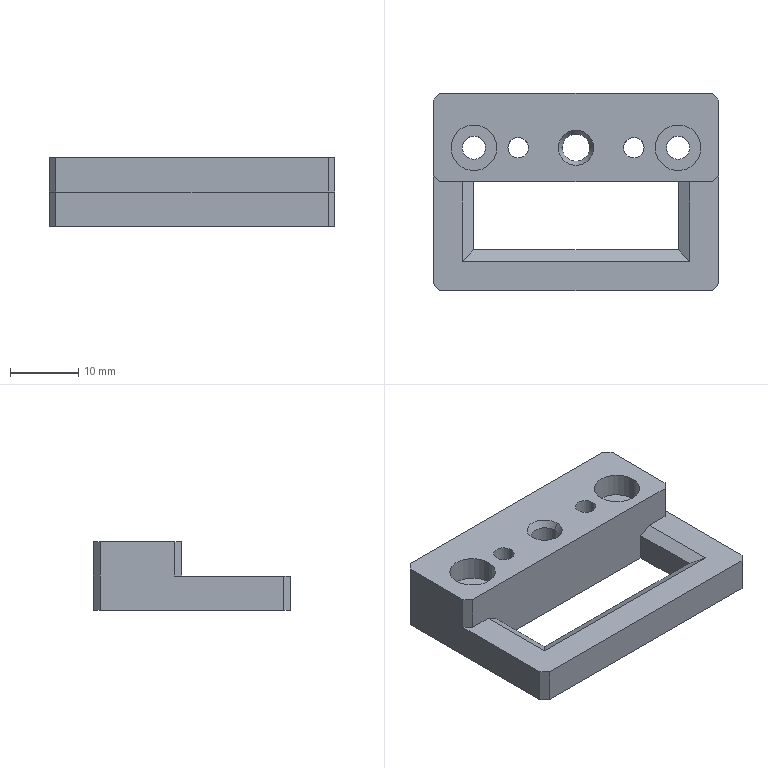Part | NX | features BREP 1 | 1 solid | 38 faces | box 42 x 29 x 10 mm | volume 6619 mm3 | plane 22 | cylinder 14 | cone 2 | commonest cylinder face diameters 3 x4 3.4 x4 6.7 x4 4 x2
STEP:
#1=CARTESIAN_POINT('',(-2.,0.,-1.));
#2=VERTEX_POINT('',#1);
#3=CARTESIAN_POINT('',(2.,0.,-1.));
#4=VERTEX_POINT('',#3);
#5=CARTESIAN_POINT('',(0.,0.,-1.));
#6=DIRECTION('',(0.,0.,1.));
#7=DIRECTION('',(1.,0.,0.));
#8=AXIS2_PLACEMENT_3D('',#5,#6,#7);
#9=CIRCLE('',#8,2.);
#10=EDGE_CURVE('',#2,#4,#9,.T.);
#11=ORIENTED_EDGE('',*,*,#10,.F.);
#12=CARTESIAN_POINT('',(-2.577,0.,0.));
#13=VERTEX_POINT('',#12);
#14=CARTESIAN_POINT('',(-2.,0.,-1.));
#15=DIRECTION('',(-0.5,0.,0.866));
#16=VECTOR('',#15,1000.);
#17=LINE('',#14,#16);
#18=EDGE_CURVE('',#13,#2,#17,.F.);
#19=ORIENTED_EDGE('',*,*,#18,.F.);
#20=CARTESIAN_POINT('',(2.577,0.,0.));
#21=VERTEX_POINT('',#20);
#22=CARTESIAN_POINT('',(0.,0.,0.));
#23=DIRECTION('',(0.,0.,-1.));
#24=DIRECTION('',(1.,0.,0.));
#25=AXIS2_PLACEMENT_3D('',#22,#23,#24);
#26=CIRCLE('',#25,2.577);
#27=EDGE_CURVE('',#21,#13,#26,.T.);
#28=ORIENTED_EDGE('',*,*,#27,.F.);
#29=CARTESIAN_POINT('',(2.,0.,-1.));
#30=DIRECTION('',(0.5,0.,0.866));
#31=VECTOR('',#30,1000.);
#32=LINE('',#29,#31);
#33=EDGE_CURVE('',#21,#4,#32,.F.);
#34=ORIENTED_EDGE('',*,*,#33,.T.);
#35=EDGE_LOOP('',(#11,#19,#28,#34));
#36=FACE_BOUND('',#35,.T.);
#37=CARTESIAN_POINT('',(0.,0.,-1.));
#38=DIRECTION('',(0.,0.,1.));
#39=DIRECTION('',(1.,0.,0.));
#40=AXIS2_PLACEMENT_3D('',#37,#38,#39);
#41=CONICAL_SURFACE('',#40,2.,0.5236);
#42=ADVANCED_FACE('',(#36),#41,.F.);
#43=CARTESIAN_POINT('',(-2.,0.,-10.));
#44=VERTEX_POINT('',#43);
#45=CARTESIAN_POINT('',(2.,0.,-10.));
#46=VERTEX_POINT('',#45);
#47=CARTESIAN_POINT('',(0.,0.,-10.));
#48=DIRECTION('',(0.,0.,1.));
#49=DIRECTION('',(1.,0.,0.));
#50=AXIS2_PLACEMENT_3D('',#47,#48,#49);
#51=CIRCLE('',#50,2.);
#52=EDGE_CURVE('',#44,#46,#51,.T.);
#53=ORIENTED_EDGE('',*,*,#52,.F.);
#54=CARTESIAN_POINT('',(-2.,0.,-29.));
#55=DIRECTION('',(0.,0.,1.));
#56=VECTOR('',#55,1000.);
#57=LINE('',#54,#56);
#58=EDGE_CURVE('',#2,#44,#57,.F.);
#59=ORIENTED_EDGE('',*,*,#58,.F.);
#60=ORIENTED_EDGE('',*,*,#10,.T.);
#61=CARTESIAN_POINT('',(2.,0.,-29.));
#62=DIRECTION('',(0.,0.,1.));
#63=VECTOR('',#62,1000.);
#64=LINE('',#61,#63);
#65=EDGE_CURVE('',#4,#46,#64,.F.);
#66=ORIENTED_EDGE('',*,*,#65,.T.);
#67=EDGE_LOOP('',(#53,#59,#60,#66));
#68=FACE_BOUND('',#67,.T.);
#69=CARTESIAN_POINT('',(0.,0.,-29.));
#70=DIRECTION('',(0.,0.,1.));
#71=DIRECTION('',(1.,0.,0.));
#72=AXIS2_PLACEMENT_3D('',#69,#70,#71);
#73=CYLINDRICAL_SURFACE('',#72,2.);
#74=ADVANCED_FACE('',(#68),#73,.F.);
#75=CARTESIAN_POINT('',(7.,0.,-10.));
#76=VERTEX_POINT('',#75);
#77=CARTESIAN_POINT('',(10.,0.,-10.));
#78=VERTEX_POINT('',#77);
#79=CARTESIAN_POINT('',(8.5,0.,-10.));
#80=DIRECTION('',(0.,0.,1.));
#81=DIRECTION('',(1.,0.,0.));
#82=AXIS2_PLACEMENT_3D('',#79,#80,#81);
#83=CIRCLE('',#82,1.5);
#84=EDGE_CURVE('',#76,#78,#83,.T.);
#85=ORIENTED_EDGE('',*,*,#84,.F.);
#86=CARTESIAN_POINT('',(7.,0.,0.));
#87=VERTEX_POINT('',#86);
#88=CARTESIAN_POINT('',(7.,0.,-19.));
#89=DIRECTION('',(0.,0.,1.));
#90=VECTOR('',#89,1000.);
#91=LINE('',#88,#90);
#92=EDGE_CURVE('',#87,#76,#91,.F.);
#93=ORIENTED_EDGE('',*,*,#92,.F.);
#94=CARTESIAN_POINT('',(10.,0.,0.));
#95=VERTEX_POINT('',#94);
#96=CARTESIAN_POINT('',(8.5,0.,0.));
#97=DIRECTION('',(0.,0.,1.));
#98=DIRECTION('',(1.,0.,0.));
#99=AXIS2_PLACEMENT_3D('',#96,#97,#98);
#100=CIRCLE('',#99,1.5);
#101=EDGE_CURVE('',#87,#95,#100,.T.);
#102=ORIENTED_EDGE('',*,*,#101,.T.);
#103=CARTESIAN_POINT('',(10.,0.,-19.));
#104=DIRECTION('',(0.,0.,1.));
#105=VECTOR('',#104,1000.);
#106=LINE('',#103,#105);
#107=EDGE_CURVE('',#95,#78,#106,.F.);
#108=ORIENTED_EDGE('',*,*,#107,.T.);
#109=EDGE_LOOP('',(#85,#93,#102,#108));
#110=FACE_BOUND('',#109,.T.);
#111=CARTESIAN_POINT('',(8.5,0.,-19.));
#112=DIRECTION('',(0.,0.,1.));
#113=DIRECTION('',(1.,0.,0.));
#114=AXIS2_PLACEMENT_3D('',#111,#112,#113);
#115=CYLINDRICAL_SURFACE('',#114,1.5);
#116=ADVANCED_FACE('',(#110),#115,.F.);
#117=CARTESIAN_POINT('',(-10.,0.,-10.));
#118=VERTEX_POINT('',#117);
#119=CARTESIAN_POINT('',(-7.,0.,-10.));
#120=VERTEX_POINT('',#119);
#121=CARTESIAN_POINT('',(-8.5,0.,-10.));
#122=DIRECTION('',(0.,0.,1.));
#123=DIRECTION('',(1.,0.,0.));
#124=AXIS2_PLACEMENT_3D('',#121,#122,#123);
#125=CIRCLE('',#124,1.5);
#126=EDGE_CURVE('',#118,#120,#125,.T.);
#127=ORIENTED_EDGE('',*,*,#126,.F.);
#128=CARTESIAN_POINT('',(-10.,0.,0.));
#129=VERTEX_POINT('',#128);
#130=CARTESIAN_POINT('',(-10.,0.,-19.));
#131=DIRECTION('',(0.,0.,1.));
#132=VECTOR('',#131,1000.);
#133=LINE('',#130,#132);
#134=EDGE_CURVE('',#129,#118,#133,.F.);
#135=ORIENTED_EDGE('',*,*,#134,.F.);
#136=CARTESIAN_POINT('',(-7.,0.,0.));
#137=VERTEX_POINT('',#136);
#138=CARTESIAN_POINT('',(-8.5,0.,0.));
#139=DIRECTION('',(0.,0.,1.));
#140=DIRECTION('',(1.,0.,0.));
#141=AXIS2_PLACEMENT_3D('',#138,#139,#140);
#142=CIRCLE('',#141,1.5);
#143=EDGE_CURVE('',#129,#137,#142,.T.);
#144=ORIENTED_EDGE('',*,*,#143,.T.);
#145=CARTESIAN_POINT('',(-7.,0.,-19.));
#146=DIRECTION('',(0.,0.,1.));
#147=VECTOR('',#146,1000.);
#148=LINE('',#145,#147);
#149=EDGE_CURVE('',#137,#120,#148,.F.);
#150=ORIENTED_EDGE('',*,*,#149,.T.);
#151=EDGE_LOOP('',(#127,#135,#144,#150));
#152=FACE_BOUND('',#151,.T.);
#153=CARTESIAN_POINT('',(-8.5,0.,-19.));
#154=DIRECTION('',(0.,0.,1.));
#155=DIRECTION('',(1.,0.,0.));
#156=AXIS2_PLACEMENT_3D('',#153,#154,#155);
#157=CYLINDRICAL_SURFACE('',#156,1.5);
#158=ADVANCED_FACE('',(#152),#157,.F.);
#159=CARTESIAN_POINT('',(-18.35,0.,-3.5));
#160=VERTEX_POINT('',#159);
#161=CARTESIAN_POINT('',(-11.65,0.,-3.5));
#162=VERTEX_POINT('',#161);
#163=CARTESIAN_POINT('',(-15.,0.,-3.5));
#164=DIRECTION('',(0.,0.,1.));
#165=DIRECTION('',(1.,0.,0.));
#166=AXIS2_PLACEMENT_3D('',#163,#164,#165);
#167=CIRCLE('',#166,3.35);
#168=EDGE_CURVE('',#160,#162,#167,.T.);
#169=ORIENTED_EDGE('',*,*,#168,.F.);
#170=CARTESIAN_POINT('',(-18.35,0.,0.));
#171=VERTEX_POINT('',#170);
#172=CARTESIAN_POINT('',(-18.35,0.,0.));
#173=DIRECTION('',(0.,0.,1.));
#174=VECTOR('',#173,1000.);
#175=LINE('',#172,#174);
#176=EDGE_CURVE('',#171,#160,#175,.F.);
#177=ORIENTED_EDGE('',*,*,#176,.F.);
#178=CARTESIAN_POINT('',(-11.65,0.,0.));
#179=VERTEX_POINT('',#178);
#180=CARTESIAN_POINT('',(-15.,0.,0.));
#181=DIRECTION('',(0.,0.,1.));
#182=DIRECTION('',(1.,0.,0.));
#183=AXIS2_PLACEMENT_3D('',#180,#181,#182);
#184=CIRCLE('',#183,3.35);
#185=EDGE_CURVE('',#171,#179,#184,.T.);
#186=ORIENTED_EDGE('',*,*,#185,.T.);
#187=CARTESIAN_POINT('',(-11.65,0.,0.));
#188=DIRECTION('',(0.,0.,1.));
#189=VECTOR('',#188,1000.);
#190=LINE('',#187,#189);
#191=EDGE_CURVE('',#179,#162,#190,.F.);
#192=ORIENTED_EDGE('',*,*,#191,.T.);
#193=EDGE_LOOP('',(#169,#177,#186,#192));
#194=FACE_BOUND('',#193,.T.);
#195=CARTESIAN_POINT('',(-15.,0.,0.));
#196=DIRECTION('',(0.,0.,1.));
#197=DIRECTION('',(1.,0.,0.));
#198=AXIS2_PLACEMENT_3D('',#195,#196,#197);
#199=CYLINDRICAL_SURFACE('',#198,3.35);
#200=ADVANCED_FACE('',(#194),#199,.F.);
#201=CARTESIAN_POINT('',(-16.7,0.,-10.));
#202=VERTEX_POINT('',#201);
#203=CARTESIAN_POINT('',(-13.3,0.,-10.));
#204=VERTEX_POINT('',#203);
#205=CARTESIAN_POINT('',(-15.,0.,-10.));
#206=DIRECTION('',(0.,0.,1.));
#207=DIRECTION('',(1.,0.,0.));
#208=AXIS2_PLACEMENT_3D('',#205,#206,#207);
#209=CIRCLE('',#208,1.7);
#210=EDGE_CURVE('',#202,#204,#209,.T.);
#211=ORIENTED_EDGE('',*,*,#210,.F.);
#212=CARTESIAN_POINT('',(-16.7,0.,-3.5));
#213=VERTEX_POINT('',#212);
#214=CARTESIAN_POINT('',(-16.7,0.,0.));
#215=DIRECTION('',(0.,0.,1.));
#216=VECTOR('',#215,1000.);
#217=LINE('',#214,#216);
#218=EDGE_CURVE('',#213,#202,#217,.F.);
#219=ORIENTED_EDGE('',*,*,#218,.F.);
#220=CARTESIAN_POINT('',(-13.3,0.,-3.5));
#221=VERTEX_POINT('',#220);
#222=CARTESIAN_POINT('',(-15.,0.,-3.5));
#223=DIRECTION('',(0.,0.,1.));
#224=DIRECTION('',(1.,0.,0.));
#225=AXIS2_PLACEMENT_3D('',#222,#223,#224);
#226=CIRCLE('',#225,1.7);
#227=EDGE_CURVE('',#213,#221,#226,.T.);
#228=ORIENTED_EDGE('',*,*,#227,.T.);
#229=CARTESIAN_POINT('',(-13.3,0.,0.));
#230=DIRECTION('',(0.,0.,1.));
#231=VECTOR('',#230,1000.);
#232=LINE('',#229,#231);
#233=EDGE_CURVE('',#221,#204,#232,.F.);
#234=ORIENTED_EDGE('',*,*,#233,.T.);
#235=EDGE_LOOP('',(#211,#219,#228,#234));
#236=FACE_BOUND('',#235,.T.);
#237=CARTESIAN_POINT('',(-15.,0.,0.));
#238=DIRECTION('',(0.,0.,1.));
#239=DIRECTION('',(1.,0.,0.));
#240=AXIS2_PLACEMENT_3D('',#237,#238,#239);
#241=CYLINDRICAL_SURFACE('',#240,1.7);
#242=ADVANCED_FACE('',(#236),#241,.F.);
#243=CARTESIAN_POINT('',(11.65,0.,-3.5));
#244=VERTEX_POINT('',#243);
#245=CARTESIAN_POINT('',(18.35,0.,-3.5));
#246=VERTEX_POINT('',#245);
#247=CARTESIAN_POINT('',(15.,0.,-3.5));
#248=DIRECTION('',(0.,0.,1.));
#249=DIRECTION('',(1.,0.,0.));
#250=AXIS2_PLACEMENT_3D('',#247,#248,#249);
#251=CIRCLE('',#250,3.35);
#252=EDGE_CURVE('',#244,#246,#251,.T.);
#253=ORIENTED_EDGE('',*,*,#252,.F.);
#254=CARTESIAN_POINT('',(11.65,0.,0.));
#255=VERTEX_POINT('',#254);
#256=CARTESIAN_POINT('',(11.65,0.,0.));
#257=DIRECTION('',(0.,0.,1.));
#258=VECTOR('',#257,1000.);
#259=LINE('',#256,#258);
#260=EDGE_CURVE('',#255,#244,#259,.F.);
#261=ORIENTED_EDGE('',*,*,#260,.F.);
#262=CARTESIAN_POINT('',(18.35,0.,0.));
#263=VERTEX_POINT('',#262);
#264=CARTESIAN_POINT('',(15.,0.,0.));
#265=DIRECTION('',(0.,0.,1.));
#266=DIRECTION('',(1.,0.,0.));
#267=AXIS2_PLACEMENT_3D('',#264,#265,#266);
#268=CIRCLE('',#267,3.35);
#269=EDGE_CURVE('',#255,#263,#268,.T.);
#270=ORIENTED_EDGE('',*,*,#269,.T.);
#271=CARTESIAN_POINT('',(18.35,0.,0.));
#272=DIRECTION('',(0.,0.,1.));
#273=VECTOR('',#272,1000.);
#274=LINE('',#271,#273);
#275=EDGE_CURVE('',#263,#246,#274,.F.);
#276=ORIENTED_EDGE('',*,*,#275,.T.);
#277=EDGE_LOOP('',(#253,#261,#270,#276));
#278=FACE_BOUND('',#277,.T.);
#279=CARTESIAN_POINT('',(15.,0.,0.));
#280=DIRECTION('',(0.,0.,1.));
#281=DIRECTION('',(1.,0.,0.));
#282=AXIS2_PLACEMENT_3D('',#279,#280,#281);
#283=CYLINDRICAL_SURFACE('',#282,3.35);
#284=ADVANCED_FACE('',(#278),#283,.F.);
#285=CARTESIAN_POINT('',(13.3,0.,-10.));
#286=VERTEX_POINT('',#285);
#287=CARTESIAN_POINT('',(16.7,0.,-10.));
#288=VERTEX_POINT('',#287);
#289=CARTESIAN_POINT('',(15.,0.,-10.));
#290=DIRECTION('',(0.,0.,1.));
#291=DIRECTION('',(1.,0.,0.));
#292=AXIS2_PLACEMENT_3D('',#289,#290,#291);
#293=CIRCLE('',#292,1.7);
#294=EDGE_CURVE('',#286,#288,#293,.T.);
#295=ORIENTED_EDGE('',*,*,#294,.F.);
#296=CARTESIAN_POINT('',(13.3,0.,-3.5));
#297=VERTEX_POINT('',#296);
#298=CARTESIAN_POINT('',(13.3,0.,0.));
#299=DIRECTION('',(0.,0.,1.));
#300=VECTOR('',#299,1000.);
#301=LINE('',#298,#300);
#302=EDGE_CURVE('',#297,#286,#301,.F.);
#303=ORIENTED_EDGE('',*,*,#302,.F.);
#304=CARTESIAN_POINT('',(16.7,0.,-3.5));
#305=VERTEX_POINT('',#304);
#306=CARTESIAN_POINT('',(15.,0.,-3.5));
#307=DIRECTION('',(0.,0.,1.));
#308=DIRECTION('',(1.,0.,0.));
#309=AXIS2_PLACEMENT_3D('',#306,#307,#308);
#310=CIRCLE('',#309,1.7);
#311=EDGE_CURVE('',#297,#305,#310,.T.);
#312=ORIENTED_EDGE('',*,*,#311,.T.);
#313=CARTESIAN_POINT('',(16.7,0.,0.));
#314=DIRECTION('',(0.,0.,1.));
#315=VECTOR('',#314,1000.);
#316=LINE('',#313,#315);
#317=EDGE_CURVE('',#305,#288,#316,.F.);
#318=ORIENTED_EDGE('',*,*,#317,.T.);
#319=EDGE_LOOP('',(#295,#303,#312,#318));
#320=FACE_BOUND('',#319,.T.);
#321=CARTESIAN_POINT('',(15.,0.,0.));
#322=DIRECTION('',(0.,0.,1.));
#323=DIRECTION('',(1.,0.,0.));
#324=AXIS2_PLACEMENT_3D('',#321,#322,#323);
#325=CYLINDRICAL_SURFACE('',#324,1.7);
#326=ADVANCED_FACE('',(#320),#325,.F.);
#327=CARTESIAN_POINT('',(20.,-21.,-10.));
#328=VERTEX_POINT('',#327);
#329=CARTESIAN_POINT('',(20.,-21.,-5.));
#330=VERTEX_POINT('',#329);
#331=CARTESIAN_POINT('',(20.,-21.,0.));
#332=DIRECTION('',(0.,0.,1.));
#333=VECTOR('',#332,1000.);
#334=LINE('',#331,#333);
#335=EDGE_CURVE('',#328,#330,#334,.T.);
#336=ORIENTED_EDGE('',*,*,#335,.T.);
#337=CARTESIAN_POINT('',(-20.,-21.,-5.));
#338=VERTEX_POINT('',#337);
#339=CARTESIAN_POINT('',(0.,-21.,-5.));
#340=DIRECTION('',(-1.,0.,0.));
#341=VECTOR('',#340,1000.);
#342=LINE('',#339,#341);
#343=EDGE_CURVE('',#330,#338,#342,.T.);
#344=ORIENTED_EDGE('',*,*,#343,.T.);
#345=CARTESIAN_POINT('',(-20.,-21.,-10.));
#346=VERTEX_POINT('',#345);
#347=CARTESIAN_POINT('',(-20.,-21.,0.));
#348=DIRECTION('',(0.,0.,-1.));
#349=VECTOR('',#348,1000.);
#350=LINE('',#347,#349);
#351=EDGE_CURVE('',#338,#346,#350,.T.);
#352=ORIENTED_EDGE('',*,*,#351,.T.);
#353=CARTESIAN_POINT('',(-21.,-21.,-10.));
#354=DIRECTION('',(1.,0.,0.));
#355=VECTOR('',#354,1000.);
#356=LINE('',#353,#355);
#357=EDGE_CURVE('',#346,#328,#356,.T.);
#358=ORIENTED_EDGE('',*,*,#357,.T.);
#359=EDGE_LOOP('',(#336,#344,#352,#358));
#360=FACE_BOUND('',#359,.T.);
#361=CARTESIAN_POINT('',(0.,-21.,0.));
#362=DIRECTION('',(0.,-1.,0.));
#363=DIRECTION('',(0.,0.,-1.));
#364=AXIS2_PLACEMENT_3D('',#361,#362,#363);
#365=PLANE('',#364);
#366=ADVANCED_FACE('',(#360),#365,.T.);
#367=CARTESIAN_POINT('',(15.,-15.,-10.));
#368=VERTEX_POINT('',#367);
#369=CARTESIAN_POINT('',(15.,-15.,-6.));
#370=VERTEX_POINT('',#369);
#371=CARTESIAN_POINT('',(15.,-15.,-16.));
#372=DIRECTION('',(0.,0.,1.));
#373=VECTOR('',#372,1000.);
#374=LINE('',#371,#373);
#375=EDGE_CURVE('',#368,#370,#374,.T.);
#376=ORIENTED_EDGE('',*,*,#375,.T.);
#377=CARTESIAN_POINT('',(15.,-5.,-6.));
#378=VERTEX_POINT('',#377);
#379=CARTESIAN_POINT('',(15.,-5.,-6.));
#380=DIRECTION('',(0.,1.,0.));
#381=VECTOR('',#380,1000.);
#382=LINE('',#379,#381);
#383=EDGE_CURVE('',#370,#378,#382,.T.);
#384=ORIENTED_EDGE('',*,*,#383,.T.);
#385=CARTESIAN_POINT('',(15.,-5.,-10.));
#386=VERTEX_POINT('',#385);
#387=CARTESIAN_POINT('',(15.,-5.,-16.));
#388=DIRECTION('',(0.,0.,1.));
#389=VECTOR('',#388,1000.);
#390=LINE('',#387,#389);
#391=EDGE_CURVE('',#386,#378,#390,.T.);
#392=ORIENTED_EDGE('',*,*,#391,.F.);
#393=CARTESIAN_POINT('',(15.,0.,-10.));
#394=DIRECTION('',(0.,1.,0.));
#395=VECTOR('',#394,1000.);
#396=LINE('',#393,#395);
#397=EDGE_CURVE('',#368,#386,#396,.T.);
#398=ORIENTED_EDGE('',*,*,#397,.F.);
#399=EDGE_LOOP('',(#376,#384,#392,#398));
#400=FACE_BOUND('',#399,.T.);
#401=CARTESIAN_POINT('',(15.,-15.,-16.));
#402=DIRECTION('',(1.,0.,0.));
#403=DIRECTION('',(0.,1.,0.));
#404=AXIS2_PLACEMENT_3D('',#401,#402,#403);
#405=PLANE('',#404);
#406=ADVANCED_FACE('',(#400),#405,.F.);
#407=CARTESIAN_POINT('',(-15.,-15.,-10.));
#408=VERTEX_POINT('',#407);
#409=CARTESIAN_POINT('',(-15.,-15.,-6.));
#410=VERTEX_POINT('',#409);
#411=CARTESIAN_POINT('',(-15.,-15.,-16.));
#412=DIRECTION('',(0.,0.,1.));
#413=VECTOR('',#412,1000.);
#414=LINE('',#411,#413);
#415=EDGE_CURVE('',#408,#410,#414,.T.);
#416=ORIENTED_EDGE('',*,*,#415,.T.);
#417=CARTESIAN_POINT('',(16.732,-15.,-6.));
#418=DIRECTION('',(1.,0.,0.));
#419=VECTOR('',#418,1000.);
#420=LINE('',#417,#419);
#421=EDGE_CURVE('',#410,#370,#420,.T.);
#422=ORIENTED_EDGE('',*,*,#421,.T.);
#423=ORIENTED_EDGE('',*,*,#375,.F.);
#424=CARTESIAN_POINT('',(0.,-15.,-10.));
#425=DIRECTION('',(1.,0.,0.));
#426=VECTOR('',#425,1000.);
#427=LINE('',#424,#426);
#428=EDGE_CURVE('',#408,#368,#427,.T.);
#429=ORIENTED_EDGE('',*,*,#428,.F.);
#430=EDGE_LOOP('',(#416,#422,#423,#429));
#431=FACE_BOUND('',#430,.T.);
#432=CARTESIAN_POINT('',(15.,-15.,-16.));
#433=DIRECTION('',(0.,-1.,0.));
#434=DIRECTION('',(0.,0.,-1.));
#435=AXIS2_PLACEMENT_3D('',#432,#433,#434);
#436=PLANE('',#435);
#437=ADVANCED_FACE('',(#431),#436,.F.);
#438=CARTESIAN_POINT('',(-15.,-5.,-10.));
#439=VERTEX_POINT('',#438);
#440=CARTESIAN_POINT('',(-15.,-5.,-6.));
#441=VERTEX_POINT('',#440);
#442=CARTESIAN_POINT('',(-15.,-5.,-16.));
#443=DIRECTION('',(0.,0.,1.));
#444=VECTOR('',#443,1000.);
#445=LINE('',#442,#444);
#446=EDGE_CURVE('',#439,#441,#445,.T.);
#447=ORIENTED_EDGE('',*,*,#446,.T.);
#448=CARTESIAN_POINT('',(-15.,-15.,-6.));
#449=DIRECTION('',(0.,-1.,0.));
#450=VECTOR('',#449,1000.);
#451=LINE('',#448,#450);
#452=EDGE_CURVE('',#441,#410,#451,.T.);
#453=ORIENTED_EDGE('',*,*,#452,.T.);
#454=ORIENTED_EDGE('',*,*,#415,.F.);
#455=CARTESIAN_POINT('',(-15.,0.,-10.));
#456=DIRECTION('',(0.,-1.,0.));
#457=VECTOR('',#456,1000.);
#458=LINE('',#455,#457);
#459=EDGE_CURVE('',#439,#408,#458,.T.);
#460=ORIENTED_EDGE('',*,*,#459,.F.);
#461=EDGE_LOOP('',(#447,#453,#454,#460));
#462=FACE_BOUND('',#461,.T.);
#463=CARTESIAN_POINT('',(-15.,-15.,-16.));
#464=DIRECTION('',(-1.,0.,0.));
#465=DIRECTION('',(0.,0.,1.));
#466=AXIS2_PLACEMENT_3D('',#463,#464,#465);
#467=PLANE('',#466);
#468=ADVANCED_FACE('',(#462),#467,.F.);
#469=CARTESIAN_POINT('',(21.,-20.,-5.));
#470=VERTEX_POINT('',#469);
#471=CARTESIAN_POINT('',(21.,-20.,-10.));
#472=VERTEX_POINT('',#471);
#473=CARTESIAN_POINT('',(21.,-20.,-10.));
#474=DIRECTION('',(0.,0.,-1.));
#475=VECTOR('',#474,1000.);
#476=LINE('',#473,#475);
#477=EDGE_CURVE('',#470,#472,#476,.T.);
#478=ORIENTED_EDGE('',*,*,#477,.F.);
#479=CARTESIAN_POINT('',(20.,-21.,-5.));
#480=DIRECTION('',(-0.7071,-0.7071,0.));
#481=VECTOR('',#480,1000.);
#482=LINE('',#479,#481);
#483=EDGE_CURVE('',#470,#330,#482,.T.);
#484=ORIENTED_EDGE('',*,*,#483,.T.);
#485=ORIENTED_EDGE('',*,*,#335,.F.);
#486=CARTESIAN_POINT('',(20.,-21.,-10.));
#487=DIRECTION('',(-0.7071,-0.7071,0.));
#488=VECTOR('',#487,1000.);
#489=LINE('',#486,#488);
#490=EDGE_CURVE('',#472,#328,#489,.T.);
#491=ORIENTED_EDGE('',*,*,#490,.F.);
#492=EDGE_LOOP('',(#478,#484,#485,#491));
#493=FACE_BOUND('',#492,.T.);
#494=CARTESIAN_POINT('',(20.,-21.,0.));
#495=DIRECTION('',(-0.7071,0.7071,0.));
#496=DIRECTION('',(0.,0.,1.));
#497=AXIS2_PLACEMENT_3D('',#494,#495,#496);
#498=PLANE('',#497);
#499=ADVANCED_FACE('',(#493),#498,.F.);
#500=ORIENTED_EDGE('',*,*,#351,.F.);
#501=CARTESIAN_POINT('',(-21.,-20.,-5.));
#502=VERTEX_POINT('',#501);
#503=CARTESIAN_POINT('',(-20.,-21.,-5.));
#504=DIRECTION('',(-0.7071,0.7071,0.));
#505=VECTOR('',#504,1000.);
#506=LINE('',#503,#505);
#507=EDGE_CURVE('',#338,#502,#506,.T.);
#508=ORIENTED_EDGE('',*,*,#507,.T.);
#509=CARTESIAN_POINT('',(-21.,-20.,-10.));
#510=VERTEX_POINT('',#509);
#511=CARTESIAN_POINT('',(-21.,-20.,-10.));
#512=DIRECTION('',(0.,0.,1.));
#513=VECTOR('',#512,1000.);
#514=LINE('',#511,#513);
#515=EDGE_CURVE('',#510,#502,#514,.T.);
#516=ORIENTED_EDGE('',*,*,#515,.F.);
#517=CARTESIAN_POINT('',(-20.,-21.,-10.));
#518=DIRECTION('',(-0.7071,0.7071,0.));
#519=VECTOR('',#518,1000.);
#520=LINE('',#517,#519);
#521=EDGE_CURVE('',#346,#510,#520,.T.);
#522=ORIENTED_EDGE('',*,*,#521,.F.);
#523=EDGE_LOOP('',(#500,#508,#516,#522));
#524=FACE_BOUND('',#523,.T.);
#525=CARTESIAN_POINT('',(-20.,-21.,0.));
#526=DIRECTION('',(0.7071,0.7071,0.));
#527=DIRECTION('',(0.,0.,-1.));
#528=AXIS2_PLACEMENT_3D('',#525,#526,#527);
#529=PLANE('',#528);
#530=ADVANCED_FACE('',(#524),#529,.F.);
#531=CARTESIAN_POINT('',(21.,-4.,0.));
#532=VERTEX_POINT('',#531);
#533=CARTESIAN_POINT('',(21.,7.,0.));
#534=VERTEX_POINT('',#533);
#535=CARTESIAN_POINT('',(21.,5.,0.));
#536=DIRECTION('',(0.,1.,0.));
#537=VECTOR('',#536,1000.);
#538=LINE('',#535,#537);
#539=EDGE_CURVE('',#532,#534,#538,.T.);
#540=ORIENTED_EDGE('',*,*,#539,.F.);
#541=CARTESIAN_POINT('',(21.,-4.,-5.));
#542=VERTEX_POINT('',#541);
#543=CARTESIAN_POINT('',(21.,-4.,-5.));
#544=DIRECTION('',(0.,0.,-1.));
#545=VECTOR('',#544,1000.);
#546=LINE('',#543,#545);
#547=EDGE_CURVE('',#532,#542,#546,.T.);
#548=ORIENTED_EDGE('',*,*,#547,.T.);
#549=CARTESIAN_POINT('',(21.,5.,-5.));
#550=DIRECTION('',(0.,-1.,0.));
#551=VECTOR('',#550,1000.);
#552=LINE('',#549,#551);
#553=EDGE_CURVE('',#542,#470,#552,.T.);
#554=ORIENTED_EDGE('',*,*,#553,.T.);
#555=ORIENTED_EDGE('',*,*,#477,.T.);
#556=CARTESIAN_POINT('',(21.,7.,-10.));
#557=VERTEX_POINT('',#556);
#558=CARTESIAN_POINT('',(21.,5.,-10.));
#559=DIRECTION('',(0.,1.,0.));
#560=VECTOR('',#559,1000.);
#561=LINE('',#558,#560);
#562=EDGE_CURVE('',#472,#557,#561,.T.);
#563=ORIENTED_EDGE('',*,*,#562,.T.);
#564=CARTESIAN_POINT('',(21.,7.,-10.));
#565=DIRECTION('',(0.,0.,1.));
#566=VECTOR('',#565,1000.);
#567=LINE('',#564,#566);
#568=EDGE_CURVE('',#557,#534,#567,.T.);
#569=ORIENTED_EDGE('',*,*,#568,.T.);
#570=EDGE_LOOP('',(#540,#548,#554,#555,#563,#569));
#571=FACE_BOUND('',#570,.T.);
#572=CARTESIAN_POINT('',(21.,5.,-10.));
#573=DIRECTION('',(1.,0.,0.));
#574=DIRECTION('',(0.,1.,0.));
#575=AXIS2_PLACEMENT_3D('',#572,#573,#574);
#576=PLANE('',#575);
#577=ADVANCED_FACE('',(#571),#576,.T.);
#578=CARTESIAN_POINT('',(-21.,-4.,-5.));
#579=VERTEX_POINT('',#578);
#580=CARTESIAN_POINT('',(-21.,-5.,-5.));
#581=DIRECTION('',(0.,-1.,0.));
#582=VECTOR('',#581,1000.);
#583=LINE('',#580,#582);
#584=EDGE_CURVE('',#579,#502,#583,.T.);
#585=ORIENTED_EDGE('',*,*,#584,.F.);
#586=CARTESIAN_POINT('',(-21.,-4.,0.));
#587=VERTEX_POINT('',#586);
#588=CARTESIAN_POINT('',(-21.,-4.,0.));
#589=DIRECTION('',(0.,0.,1.));
#590=VECTOR('',#589,1000.);
#591=LINE('',#588,#590);
#592=EDGE_CURVE('',#579,#587,#591,.T.);
#593=ORIENTED_EDGE('',*,*,#592,.T.);
#594=CARTESIAN_POINT('',(-21.,7.,0.));
#595=VERTEX_POINT('',#594);
#596=CARTESIAN_POINT('',(-21.,5.,0.));
#597=DIRECTION('',(0.,-1.,0.));
#598=VECTOR('',#597,1000.);
#599=LINE('',#596,#598);
#600=EDGE_CURVE('',#595,#587,#599,.T.);
#601=ORIENTED_EDGE('',*,*,#600,.F.);
#602=CARTESIAN_POINT('',(-21.,7.,-10.));
#603=VERTEX_POINT('',#602);
#604=CARTESIAN_POINT('',(-21.,7.,-10.));
#605=DIRECTION('',(0.,0.,-1.));
#606=VECTOR('',#605,1000.);
#607=LINE('',#604,#606);
#608=EDGE_CURVE('',#595,#603,#607,.T.);
#609=ORIENTED_EDGE('',*,*,#608,.T.);
#610=CARTESIAN_POINT('',(-21.,5.,-10.));
#611=DIRECTION('',(0.,-1.,0.));
#612=VECTOR('',#611,1000.);
#613=LINE('',#610,#612);
#614=EDGE_CURVE('',#603,#510,#613,.T.);
#615=ORIENTED_EDGE('',*,*,#614,.T.);
#616=ORIENTED_EDGE('',*,*,#515,.T.);
#617=EDGE_LOOP('',(#585,#593,#601,#609,#615,#616));
#618=FACE_BOUND('',#617,.T.);
#619=CARTESIAN_POINT('',(-21.,5.,-10.));
#620=DIRECTION('',(-1.,0.,0.));
#621=DIRECTION('',(0.,1.,0.));
#622=AXIS2_PLACEMENT_3D('',#619,#620,#621);
#623=PLANE('',#622);
#624=ADVANCED_FACE('',(#618),#623,.T.);
#625=CARTESIAN_POINT('',(20.,8.,-10.));
#626=VERTEX_POINT('',#625);
#627=CARTESIAN_POINT('',(-20.,8.,-10.));
#628=VERTEX_POINT('',#627);
#629=CARTESIAN_POINT('',(-21.,8.,-10.));
#630=DIRECTION('',(-1.,0.,0.));
#631=VECTOR('',#630,1000.);
#632=LINE('',#629,#631);
#633=EDGE_CURVE('',#626,#628,#632,.T.);
#634=ORIENTED_EDGE('',*,*,#633,.F.);
#635=CARTESIAN_POINT('',(20.,8.,-10.));
#636=DIRECTION('',(0.7071,-0.7071,0.));
#637=VECTOR('',#636,1000.);
#638=LINE('',#635,#637);
#639=EDGE_CURVE('',#626,#557,#638,.T.);
#640=ORIENTED_EDGE('',*,*,#639,.T.);
#641=ORIENTED_EDGE('',*,*,#562,.F.);
#642=ORIENTED_EDGE('',*,*,#490,.T.);
#643=ORIENTED_EDGE('',*,*,#357,.F.);
#644=ORIENTED_EDGE('',*,*,#521,.T.);
#645=ORIENTED_EDGE('',*,*,#614,.F.);
#646=CARTESIAN_POINT('',(-20.,8.,-10.));
#647=DIRECTION('',(0.7071,0.7071,0.));
#648=VECTOR('',#647,1000.);
#649=LINE('',#646,#648);
#650=EDGE_CURVE('',#603,#628,#649,.T.);
#651=ORIENTED_EDGE('',*,*,#650,.T.);
#652=EDGE_LOOP('',(#634,#640,#641,#642,#643,#644,#645,#651));
#653=FACE_BOUND('',#652,.T.);
#654=CARTESIAN_POINT('',(0.,0.,-10.));
#655=DIRECTION('',(0.,0.,1.));
#656=DIRECTION('',(1.,0.,0.));
#657=AXIS2_PLACEMENT_3D('',#654,#655,#656);
#658=CIRCLE('',#657,2.);
#659=EDGE_CURVE('',#46,#44,#658,.T.);
#660=ORIENTED_EDGE('',*,*,#659,.T.);
#661=ORIENTED_EDGE('',*,*,#52,.T.);
#662=EDGE_LOOP('',(#660,#661));
#663=FACE_BOUND('',#662,.T.);
#664=ORIENTED_EDGE('',*,*,#428,.T.);
#665=ORIENTED_EDGE('',*,*,#397,.T.);
#666=CARTESIAN_POINT('',(0.,-5.,-10.));
#667=DIRECTION('',(-1.,0.,0.));
#668=VECTOR('',#667,1000.);
#669=LINE('',#666,#668);
#670=EDGE_CURVE('',#386,#439,#669,.T.);
#671=ORIENTED_EDGE('',*,*,#670,.T.);
#672=ORIENTED_EDGE('',*,*,#459,.T.);
#673=EDGE_LOOP('',(#664,#665,#671,#672));
#674=FACE_BOUND('',#673,.T.);
#675=CARTESIAN_POINT('',(8.5,0.,-10.));
#676=DIRECTION('',(0.,0.,1.));
#677=DIRECTION('',(1.,0.,0.));
#678=AXIS2_PLACEMENT_3D('',#675,#676,#677);
#679=CIRCLE('',#678,1.5);
#680=EDGE_CURVE('',#78,#76,#679,.T.);
#681=ORIENTED_EDGE('',*,*,#680,.T.);
#682=ORIENTED_EDGE('',*,*,#84,.T.);
#683=EDGE_LOOP('',(#681,#682));
#684=FACE_BOUND('',#683,.T.);
#685=CARTESIAN_POINT('',(-8.5,0.,-10.));
#686=DIRECTION('',(0.,0.,1.));
#687=DIRECTION('',(1.,0.,0.));
#688=AXIS2_PLACEMENT_3D('',#685,#686,#687);
#689=CIRCLE('',#688,1.5);
#690=EDGE_CURVE('',#120,#118,#689,.T.);
#691=ORIENTED_EDGE('',*,*,#690,.T.);
#692=ORIENTED_EDGE('',*,*,#126,.T.);
#693=EDGE_LOOP('',(#691,#692));
#694=FACE_BOUND('',#693,.T.);
#695=CARTESIAN_POINT('',(-15.,0.,-10.));
#696=DIRECTION('',(0.,0.,1.));
#697=DIRECTION('',(1.,0.,0.));
#698=AXIS2_PLACEMENT_3D('',#695,#696,#697);
#699=CIRCLE('',#698,1.7);
#700=EDGE_CURVE('',#204,#202,#699,.T.);
#701=ORIENTED_EDGE('',*,*,#700,.T.);
#702=ORIENTED_EDGE('',*,*,#210,.T.);
#703=EDGE_LOOP('',(#701,#702));
#704=FACE_BOUND('',#703,.T.);
#705=CARTESIAN_POINT('',(15.,0.,-10.));
#706=DIRECTION('',(0.,0.,1.));
#707=DIRECTION('',(1.,0.,0.));
#708=AXIS2_PLACEMENT_3D('',#705,#706,#707);
#709=CIRCLE('',#708,1.7);
#710=EDGE_CURVE('',#288,#286,#709,.T.);
#711=ORIENTED_EDGE('',*,*,#710,.T.);
#712=ORIENTED_EDGE('',*,*,#294,.T.);
#713=EDGE_LOOP('',(#711,#712));
#714=FACE_BOUND('',#713,.T.);
#715=CARTESIAN_POINT('',(0.,0.,-10.));
#716=DIRECTION('',(0.,0.,1.));
#717=DIRECTION('',(1.,0.,0.));
#718=AXIS2_PLACEMENT_3D('',#715,#716,#717);
#719=PLANE('',#718);
#720=ADVANCED_FACE('',(#653,#663,#674,#684,#694,#704,#714),#719,.F.);
#721=ORIENTED_EDGE('',*,*,#600,.T.);
#722=CARTESIAN_POINT('',(-20.,-5.,0.));
#723=VERTEX_POINT('',#722);
#724=CARTESIAN_POINT('',(-12.5,-12.5,0.));
#725=DIRECTION('',(0.7071,-0.7071,0.));
#726=VECTOR('',#725,1000.);
#727=LINE('',#724,#726);
#728=EDGE_CURVE('',#587,#723,#727,.T.);
#729=ORIENTED_EDGE('',*,*,#728,.T.);
#730=CARTESIAN_POINT('',(20.,-5.,0.));
#731=VERTEX_POINT('',#730);
#732=CARTESIAN_POINT('',(15.,-5.,0.));
#733=DIRECTION('',(-1.,0.,0.));
#734=VECTOR('',#733,1000.);
#735=LINE('',#732,#734);
#736=EDGE_CURVE('',#731,#723,#735,.T.);
#737=ORIENTED_EDGE('',*,*,#736,.F.);
#738=CARTESIAN_POINT('',(12.5,-12.5,0.));
#739=DIRECTION('',(0.7071,0.7071,0.));
#740=VECTOR('',#739,1000.);
#741=LINE('',#738,#740);
#742=EDGE_CURVE('',#731,#532,#741,.T.);
#743=ORIENTED_EDGE('',*,*,#742,.T.);
#744=ORIENTED_EDGE('',*,*,#539,.T.);
#745=CARTESIAN_POINT('',(20.,8.,0.));
#746=VERTEX_POINT('',#745);
#747=CARTESIAN_POINT('',(14.,14.,0.));
#748=DIRECTION('',(-0.7071,0.7071,0.));
#749=VECTOR('',#748,1000.);
#750=LINE('',#747,#749);
#751=EDGE_CURVE('',#534,#746,#750,.T.);
#752=ORIENTED_EDGE('',*,*,#751,.T.);
#753=CARTESIAN_POINT('',(-20.,8.,0.));
#754=VERTEX_POINT('',#753);
#755=CARTESIAN_POINT('',(-21.,8.,0.));
#756=DIRECTION('',(1.,0.,0.));
#757=VECTOR('',#756,1000.);
#758=LINE('',#755,#757);
#759=EDGE_CURVE('',#754,#746,#758,.T.);
#760=ORIENTED_EDGE('',*,*,#759,.F.);
#761=CARTESIAN_POINT('',(-14.,14.,0.));
#762=DIRECTION('',(-0.7071,-0.7071,0.));
#763=VECTOR('',#762,1000.);
#764=LINE('',#761,#763);
#765=EDGE_CURVE('',#754,#595,#764,.T.);
#766=ORIENTED_EDGE('',*,*,#765,.T.);
#767=EDGE_LOOP('',(#721,#729,#737,#743,#744,#752,#760,#766));
#768=FACE_BOUND('',#767,.T.);
#769=ORIENTED_EDGE('',*,*,#27,.T.);
#770=CARTESIAN_POINT('',(0.,0.,0.));
#771=DIRECTION('',(0.,0.,-1.));
#772=DIRECTION('',(1.,0.,0.));
#773=AXIS2_PLACEMENT_3D('',#770,#771,#772);
#774=CIRCLE('',#773,2.577);
#775=EDGE_CURVE('',#13,#21,#774,.T.);
#776=ORIENTED_EDGE('',*,*,#775,.T.);
#777=EDGE_LOOP('',(#769,#776));
#778=FACE_BOUND('',#777,.T.);
#779=CARTESIAN_POINT('',(8.5,0.,0.));
#780=DIRECTION('',(0.,0.,1.));
#781=DIRECTION('',(1.,0.,0.));
#782=AXIS2_PLACEMENT_3D('',#779,#780,#781);
#783=CIRCLE('',#782,1.5);
#784=EDGE_CURVE('',#95,#87,#783,.T.);
#785=ORIENTED_EDGE('',*,*,#784,.F.);
#786=ORIENTED_EDGE('',*,*,#101,.F.);
#787=EDGE_LOOP('',(#785,#786));
#788=FACE_BOUND('',#787,.T.);
#789=CARTESIAN_POINT('',(-8.5,0.,0.));
#790=DIRECTION('',(0.,0.,1.));
#791=DIRECTION('',(1.,0.,0.));
#792=AXIS2_PLACEMENT_3D('',#789,#790,#791);
#793=CIRCLE('',#792,1.5);
#794=EDGE_CURVE('',#137,#129,#793,.T.);
#795=ORIENTED_EDGE('',*,*,#794,.F.);
#796=ORIENTED_EDGE('',*,*,#143,.F.);
#797=EDGE_LOOP('',(#795,#796));
#798=FACE_BOUND('',#797,.T.);
#799=CARTESIAN_POINT('',(-15.,0.,0.));
#800=DIRECTION('',(0.,0.,1.));
#801=DIRECTION('',(1.,0.,0.));
#802=AXIS2_PLACEMENT_3D('',#799,#800,#801);
#803=CIRCLE('',#802,3.35);
#804=EDGE_CURVE('',#179,#171,#803,.T.);
#805=ORIENTED_EDGE('',*,*,#804,.F.);
#806=ORIENTED_EDGE('',*,*,#185,.F.);
#807=EDGE_LOOP('',(#805,#806));
#808=FACE_BOUND('',#807,.T.);
#809=CARTESIAN_POINT('',(15.,0.,0.));
#810=DIRECTION('',(0.,0.,1.));
#811=DIRECTION('',(1.,0.,0.));
#812=AXIS2_PLACEMENT_3D('',#809,#810,#811);
#813=CIRCLE('',#812,3.35);
#814=EDGE_CURVE('',#263,#255,#813,.T.);
#815=ORIENTED_EDGE('',*,*,#814,.F.);
#816=ORIENTED_EDGE('',*,*,#269,.F.);
#817=EDGE_LOOP('',(#815,#816));
#818=FACE_BOUND('',#817,.T.);
#819=CARTESIAN_POINT('',(0.,0.,0.));
#820=DIRECTION('',(0.,0.,1.));
#821=DIRECTION('',(1.,0.,0.));
#822=AXIS2_PLACEMENT_3D('',#819,#820,#821);
#823=PLANE('',#822);
#824=ADVANCED_FACE('',(#768,#778,#788,#798,#808,#818),#823,.T.);
#825=ORIENTED_EDGE('',*,*,#302,.T.);
#826=ORIENTED_EDGE('',*,*,#710,.F.);
#827=ORIENTED_EDGE('',*,*,#317,.F.);
#828=CARTESIAN_POINT('',(15.,0.,-3.5));
#829=DIRECTION('',(0.,0.,1.));
#830=DIRECTION('',(1.,0.,0.));
#831=AXIS2_PLACEMENT_3D('',#828,#829,#830);
#832=CIRCLE('',#831,1.7);
#833=EDGE_CURVE('',#305,#297,#832,.T.);
#834=ORIENTED_EDGE('',*,*,#833,.T.);
#835=EDGE_LOOP('',(#825,#826,#827,#834));
#836=FACE_BOUND('',#835,.T.);
#837=CARTESIAN_POINT('',(15.,0.,0.));
#838=DIRECTION('',(0.,0.,1.));
#839=DIRECTION('',(1.,0.,0.));
#840=AXIS2_PLACEMENT_3D('',#837,#838,#839);
#841=CYLINDRICAL_SURFACE('',#840,1.7);
#842=ADVANCED_FACE('',(#836),#841,.F.);
#843=CARTESIAN_POINT('',(15.,0.,-3.5));
#844=DIRECTION('',(0.,0.,1.));
#845=DIRECTION('',(1.,0.,0.));
#846=AXIS2_PLACEMENT_3D('',#843,#844,#845);
#847=CIRCLE('',#846,3.35);
#848=EDGE_CURVE('',#246,#244,#847,.T.);
#849=ORIENTED_EDGE('',*,*,#848,.T.);
#850=ORIENTED_EDGE('',*,*,#252,.T.);
#851=EDGE_LOOP('',(#849,#850));
#852=FACE_BOUND('',#851,.T.);
#853=ORIENTED_EDGE('',*,*,#833,.F.);
#854=ORIENTED_EDGE('',*,*,#311,.F.);
#855=EDGE_LOOP('',(#853,#854));
#856=FACE_BOUND('',#855,.T.);
#857=CARTESIAN_POINT('',(16.7,0.,-3.5));
#858=DIRECTION('',(0.,0.,-1.));
#859=DIRECTION('',(0.,-1.,0.));
#860=AXIS2_PLACEMENT_3D('',#857,#858,#859);
#861=PLANE('',#860);
#862=ADVANCED_FACE('',(#852,#856),#861,.F.);
#863=ORIENTED_EDGE('',*,*,#260,.T.);
#864=ORIENTED_EDGE('',*,*,#848,.F.);
#865=ORIENTED_EDGE('',*,*,#275,.F.);
#866=ORIENTED_EDGE('',*,*,#814,.T.);
#867=EDGE_LOOP('',(#863,#864,#865,#866));
#868=FACE_BOUND('',#867,.T.);
#869=CARTESIAN_POINT('',(15.,0.,0.));
#870=DIRECTION('',(0.,0.,1.));
#871=DIRECTION('',(1.,0.,0.));
#872=AXIS2_PLACEMENT_3D('',#869,#870,#871);
#873=CYLINDRICAL_SURFACE('',#872,3.35);
#874=ADVANCED_FACE('',(#868),#873,.F.);
#875=ORIENTED_EDGE('',*,*,#218,.T.);
#876=ORIENTED_EDGE('',*,*,#700,.F.);
#877=ORIENTED_EDGE('',*,*,#233,.F.);
#878=CARTESIAN_POINT('',(-15.,0.,-3.5));
#879=DIRECTION('',(0.,0.,1.));
#880=DIRECTION('',(1.,0.,0.));
#881=AXIS2_PLACEMENT_3D('',#878,#879,#880);
#882=CIRCLE('',#881,1.7);
#883=EDGE_CURVE('',#221,#213,#882,.T.);
#884=ORIENTED_EDGE('',*,*,#883,.T.);
#885=EDGE_LOOP('',(#875,#876,#877,#884));
#886=FACE_BOUND('',#885,.T.);
#887=CARTESIAN_POINT('',(-15.,0.,0.));
#888=DIRECTION('',(0.,0.,1.));
#889=DIRECTION('',(1.,0.,0.));
#890=AXIS2_PLACEMENT_3D('',#887,#888,#889);
#891=CYLINDRICAL_SURFACE('',#890,1.7);
#892=ADVANCED_FACE('',(#886),#891,.F.);
#893=CARTESIAN_POINT('',(-15.,0.,-3.5));
#894=DIRECTION('',(0.,0.,1.));
#895=DIRECTION('',(1.,0.,0.));
#896=AXIS2_PLACEMENT_3D('',#893,#894,#895);
#897=CIRCLE('',#896,3.35);
#898=EDGE_CURVE('',#162,#160,#897,.T.);
#899=ORIENTED_EDGE('',*,*,#898,.T.);
#900=ORIENTED_EDGE('',*,*,#168,.T.);
#901=EDGE_LOOP('',(#899,#900));
#902=FACE_BOUND('',#901,.T.);
#903=ORIENTED_EDGE('',*,*,#883,.F.);
#904=ORIENTED_EDGE('',*,*,#227,.F.);
#905=EDGE_LOOP('',(#903,#904));
#906=FACE_BOUND('',#905,.T.);
#907=CARTESIAN_POINT('',(-13.3,0.,-3.5));
#908=DIRECTION('',(0.,0.,-1.));
#909=DIRECTION('',(0.,-1.,0.));
#910=AXIS2_PLACEMENT_3D('',#907,#908,#909);
#911=PLANE('',#910);
#912=ADVANCED_FACE('',(#902,#906),#911,.F.);
#913=ORIENTED_EDGE('',*,*,#176,.T.);
#914=ORIENTED_EDGE('',*,*,#898,.F.);
#915=ORIENTED_EDGE('',*,*,#191,.F.);
#916=ORIENTED_EDGE('',*,*,#804,.T.);
#917=EDGE_LOOP('',(#913,#914,#915,#916));
#918=FACE_BOUND('',#917,.T.);
#919=CARTESIAN_POINT('',(-15.,0.,0.));
#920=DIRECTION('',(0.,0.,1.));
#921=DIRECTION('',(1.,0.,0.));
#922=AXIS2_PLACEMENT_3D('',#919,#920,#921);
#923=CYLINDRICAL_SURFACE('',#922,3.35);
#924=ADVANCED_FACE('',(#918),#923,.F.);
#925=ORIENTED_EDGE('',*,*,#134,.T.);
#926=ORIENTED_EDGE('',*,*,#690,.F.);
#927=ORIENTED_EDGE('',*,*,#149,.F.);
#928=ORIENTED_EDGE('',*,*,#794,.T.);
#929=EDGE_LOOP('',(#925,#926,#927,#928));
#930=FACE_BOUND('',#929,.T.);
#931=CARTESIAN_POINT('',(-8.5,0.,-19.));
#932=DIRECTION('',(0.,0.,1.));
#933=DIRECTION('',(1.,0.,0.));
#934=AXIS2_PLACEMENT_3D('',#931,#932,#933);
#935=CYLINDRICAL_SURFACE('',#934,1.5);
#936=ADVANCED_FACE('',(#930),#935,.F.);
#937=ORIENTED_EDGE('',*,*,#92,.T.);
#938=ORIENTED_EDGE('',*,*,#680,.F.);
#939=ORIENTED_EDGE('',*,*,#107,.F.);
#940=ORIENTED_EDGE('',*,*,#784,.T.);
#941=EDGE_LOOP('',(#937,#938,#939,#940));
#942=FACE_BOUND('',#941,.T.);
#943=CARTESIAN_POINT('',(8.5,0.,-19.));
#944=DIRECTION('',(0.,0.,1.));
#945=DIRECTION('',(1.,0.,0.));
#946=AXIS2_PLACEMENT_3D('',#943,#944,#945);
#947=CYLINDRICAL_SURFACE('',#946,1.5);
#948=ADVANCED_FACE('',(#942),#947,.F.);
#949=ORIENTED_EDGE('',*,*,#736,.T.);
#950=CARTESIAN_POINT('',(-20.,-5.,-5.));
#951=VERTEX_POINT('',#950);
#952=CARTESIAN_POINT('',(-20.,-5.,-5.));
#953=DIRECTION('',(0.,0.,-1.));
#954=VECTOR('',#953,1000.);
#955=LINE('',#952,#954);
#956=EDGE_CURVE('',#723,#951,#955,.T.);
#957=ORIENTED_EDGE('',*,*,#956,.T.);
#958=CARTESIAN_POINT('',(-16.732,-5.,-5.));
#959=VERTEX_POINT('',#958);
#960=CARTESIAN_POINT('',(-21.,-5.,-5.));
#961=DIRECTION('',(-1.,0.,0.));
#962=VECTOR('',#961,1000.);
#963=LINE('',#960,#962);
#964=EDGE_CURVE('',#959,#951,#963,.T.);
#965=ORIENTED_EDGE('',*,*,#964,.F.);
#966=CARTESIAN_POINT('',(11.83,-5.,-21.49));
#967=DIRECTION('',(0.866,0.,-0.5));
#968=VECTOR('',#967,1000.);
#969=LINE('',#966,#968);
#970=EDGE_CURVE('',#959,#441,#969,.T.);
#971=ORIENTED_EDGE('',*,*,#970,.T.);
#972=ORIENTED_EDGE('',*,*,#446,.F.);
#973=ORIENTED_EDGE('',*,*,#670,.F.);
#974=ORIENTED_EDGE('',*,*,#391,.T.);
#975=CARTESIAN_POINT('',(16.732,-5.,-5.));
#976=VERTEX_POINT('',#975);
#977=CARTESIAN_POINT('',(10.67,-5.,-8.5));
#978=DIRECTION('',(0.866,0.,0.5));
#979=VECTOR('',#978,1000.);
#980=LINE('',#977,#979);
#981=EDGE_CURVE('',#378,#976,#980,.T.);
#982=ORIENTED_EDGE('',*,*,#981,.T.);
#983=CARTESIAN_POINT('',(20.,-5.,-5.));
#984=VERTEX_POINT('',#983);
#985=CARTESIAN_POINT('',(-21.,-5.,-5.));
#986=DIRECTION('',(-1.,0.,0.));
#987=VECTOR('',#986,1000.);
#988=LINE('',#985,#987);
#989=EDGE_CURVE('',#984,#976,#988,.T.);
#990=ORIENTED_EDGE('',*,*,#989,.F.);
#991=CARTESIAN_POINT('',(20.,-5.,0.));
#992=DIRECTION('',(0.,0.,1.));
#993=VECTOR('',#992,1000.);
#994=LINE('',#991,#993);
#995=EDGE_CURVE('',#984,#731,#994,.T.);
#996=ORIENTED_EDGE('',*,*,#995,.T.);
#997=EDGE_LOOP('',(#949,#957,#965,#971,#972,#973,#974,#982,#990,#996));
#998=FACE_BOUND('',#997,.T.);
#999=CARTESIAN_POINT('',(15.,-5.,-16.));
#1000=DIRECTION('',(0.,1.,0.));
#1001=DIRECTION('',(1.,0.,0.));
#1002=AXIS2_PLACEMENT_3D('',#999,#1000,#1001);
#1003=PLANE('',#1002);
#1004=ADVANCED_FACE('',(#998),#1003,.F.);
#1005=ORIENTED_EDGE('',*,*,#58,.T.);
#1006=ORIENTED_EDGE('',*,*,#659,.F.);
#1007=ORIENTED_EDGE('',*,*,#65,.F.);
#1008=CARTESIAN_POINT('',(0.,0.,-1.));
#1009=DIRECTION('',(0.,0.,1.));
#1010=DIRECTION('',(1.,0.,0.));
#1011=AXIS2_PLACEMENT_3D('',#1008,#1009,#1010);
#1012=CIRCLE('',#1011,2.);
#1013=EDGE_CURVE('',#4,#2,#1012,.T.);
#1014=ORIENTED_EDGE('',*,*,#1013,.T.);
#1015=EDGE_LOOP('',(#1005,#1006,#1007,#1014));
#1016=FACE_BOUND('',#1015,.T.);
#1017=CARTESIAN_POINT('',(0.,0.,-29.));
#1018=DIRECTION('',(0.,0.,1.));
#1019=DIRECTION('',(1.,0.,0.));
#1020=AXIS2_PLACEMENT_3D('',#1017,#1018,#1019);
#1021=CYLINDRICAL_SURFACE('',#1020,2.);
#1022=ADVANCED_FACE('',(#1016),#1021,.F.);
#1023=ORIENTED_EDGE('',*,*,#18,.T.);
#1024=ORIENTED_EDGE('',*,*,#1013,.F.);
#1025=ORIENTED_EDGE('',*,*,#33,.F.);
#1026=ORIENTED_EDGE('',*,*,#775,.F.);
#1027=EDGE_LOOP('',(#1023,#1024,#1025,#1026));
#1028=FACE_BOUND('',#1027,.T.);
#1029=CARTESIAN_POINT('',(0.,0.,-1.));
#1030=DIRECTION('',(0.,0.,1.));
#1031=DIRECTION('',(1.,0.,0.));
#1032=AXIS2_PLACEMENT_3D('',#1029,#1030,#1031);
#1033=CONICAL_SURFACE('',#1032,2.,0.5236);
#1034=ADVANCED_FACE('',(#1028),#1033,.F.);
#1035=ORIENTED_EDGE('',*,*,#759,.T.);
#1036=CARTESIAN_POINT('',(20.,8.,0.));
#1037=DIRECTION('',(0.,0.,-1.));
#1038=VECTOR('',#1037,1000.);
#1039=LINE('',#1036,#1038);
#1040=EDGE_CURVE('',#746,#626,#1039,.T.);
#1041=ORIENTED_EDGE('',*,*,#1040,.T.);
#1042=ORIENTED_EDGE('',*,*,#633,.T.);
#1043=CARTESIAN_POINT('',(-20.,8.,0.));
#1044=DIRECTION('',(0.,0.,1.));
#1045=VECTOR('',#1044,1000.);
#1046=LINE('',#1043,#1045);
#1047=EDGE_CURVE('',#628,#754,#1046,.T.);
#1048=ORIENTED_EDGE('',*,*,#1047,.T.);
#1049=EDGE_LOOP('',(#1035,#1041,#1042,#1048));
#1050=FACE_BOUND('',#1049,.T.);
#1051=CARTESIAN_POINT('',(0.,8.,0.));
#1052=DIRECTION('',(0.,1.,0.));
#1053=DIRECTION('',(1.,0.,0.));
#1054=AXIS2_PLACEMENT_3D('',#1051,#1052,#1053);
#1055=PLANE('',#1054);
#1056=ADVANCED_FACE('',(#1050),#1055,.T.);
#1057=ORIENTED_EDGE('',*,*,#751,.F.);
#1058=ORIENTED_EDGE('',*,*,#568,.F.);
#1059=ORIENTED_EDGE('',*,*,#639,.F.);
#1060=ORIENTED_EDGE('',*,*,#1040,.F.);
#1061=EDGE_LOOP('',(#1057,#1058,#1059,#1060));
#1062=FACE_BOUND('',#1061,.T.);
#1063=CARTESIAN_POINT('',(20.,8.,0.));
#1064=DIRECTION('',(-0.7071,-0.7071,0.));
#1065=DIRECTION('',(-0.7071,0.7071,0.));
#1066=AXIS2_PLACEMENT_3D('',#1063,#1064,#1065);
#1067=PLANE('',#1066);
#1068=ADVANCED_FACE('',(#1062),#1067,.F.);
#1069=ORIENTED_EDGE('',*,*,#650,.F.);
#1070=ORIENTED_EDGE('',*,*,#608,.F.);
#1071=ORIENTED_EDGE('',*,*,#765,.F.);
#1072=ORIENTED_EDGE('',*,*,#1047,.F.);
#1073=EDGE_LOOP('',(#1069,#1070,#1071,#1072));
#1074=FACE_BOUND('',#1073,.T.);
#1075=CARTESIAN_POINT('',(-20.,8.,0.));
#1076=DIRECTION('',(0.7071,-0.7071,0.));
#1077=DIRECTION('',(0.,0.,-1.));
#1078=AXIS2_PLACEMENT_3D('',#1075,#1076,#1077);
#1079=PLANE('',#1078);
#1080=ADVANCED_FACE('',(#1074),#1079,.F.);
#1081=CARTESIAN_POINT('',(16.732,-16.732,-5.));
#1082=VERTEX_POINT('',#1081);
#1083=CARTESIAN_POINT('',(-16.732,-16.732,-5.));
#1084=VERTEX_POINT('',#1083);
#1085=CARTESIAN_POINT('',(-16.732,-16.732,-5.));
#1086=DIRECTION('',(-1.,0.,0.));
#1087=VECTOR('',#1086,1000.);
#1088=LINE('',#1085,#1087);
#1089=EDGE_CURVE('',#1082,#1084,#1088,.T.);
#1090=ORIENTED_EDGE('',*,*,#1089,.T.);
#1091=CARTESIAN_POINT('',(-16.732,-5.,-5.));
#1092=DIRECTION('',(0.,1.,0.));
#1093=VECTOR('',#1092,1000.);
#1094=LINE('',#1091,#1093);
#1095=EDGE_CURVE('',#1084,#959,#1094,.T.);
#1096=ORIENTED_EDGE('',*,*,#1095,.T.);
#1097=ORIENTED_EDGE('',*,*,#964,.T.);
#1098=CARTESIAN_POINT('',(-21.,-4.,-5.));
#1099=DIRECTION('',(-0.7071,0.7071,0.));
#1100=VECTOR('',#1099,1000.);
#1101=LINE('',#1098,#1100);
#1102=EDGE_CURVE('',#951,#579,#1101,.T.);
#1103=ORIENTED_EDGE('',*,*,#1102,.T.);
#1104=ORIENTED_EDGE('',*,*,#584,.T.);
#1105=ORIENTED_EDGE('',*,*,#507,.F.);
#1106=ORIENTED_EDGE('',*,*,#343,.F.);
#1107=ORIENTED_EDGE('',*,*,#483,.F.);
#1108=ORIENTED_EDGE('',*,*,#553,.F.);
#1109=CARTESIAN_POINT('',(20.,-5.,-5.));
#1110=DIRECTION('',(-0.7071,-0.7071,0.));
#1111=VECTOR('',#1110,1000.);
#1112=LINE('',#1109,#1111);
#1113=EDGE_CURVE('',#542,#984,#1112,.T.);
#1114=ORIENTED_EDGE('',*,*,#1113,.T.);
#1115=ORIENTED_EDGE('',*,*,#989,.T.);
#1116=CARTESIAN_POINT('',(16.732,-15.,-5.));
#1117=DIRECTION('',(0.,-1.,0.));
#1118=VECTOR('',#1117,1000.);
#1119=LINE('',#1116,#1118);
#1120=EDGE_CURVE('',#976,#1082,#1119,.T.);
#1121=ORIENTED_EDGE('',*,*,#1120,.T.);
#1122=EDGE_LOOP('',(#1090,#1096,#1097,#1103,#1104,#1105,#1106,#1107,#1108,#1114,#1115,#1121));
#1123=FACE_BOUND('',#1122,.T.);
#1124=CARTESIAN_POINT('',(0.,0.,-5.));
#1125=DIRECTION('',(0.,0.,1.));
#1126=DIRECTION('',(1.,0.,0.));
#1127=AXIS2_PLACEMENT_3D('',#1124,#1125,#1126);
#1128=PLANE('',#1127);
#1129=ADVANCED_FACE('',(#1123),#1128,.T.);
#1130=ORIENTED_EDGE('',*,*,#1095,.F.);
#1131=CARTESIAN_POINT('',(-9.561,-9.561,-9.14));
#1132=DIRECTION('',(0.6547,0.6547,-0.378));
#1133=VECTOR('',#1132,1000.);
#1134=LINE('',#1131,#1133);
#1135=EDGE_CURVE('',#1084,#410,#1134,.T.);
#1136=ORIENTED_EDGE('',*,*,#1135,.T.);
#1137=ORIENTED_EDGE('',*,*,#452,.F.);
#1138=ORIENTED_EDGE('',*,*,#970,.F.);
#1139=EDGE_LOOP('',(#1130,#1136,#1137,#1138));
#1140=FACE_BOUND('',#1139,.T.);
#1141=CARTESIAN_POINT('',(-16.732,0.,-5.));
#1142=DIRECTION('',(0.5,0.,0.866));
#1143=DIRECTION('',(0.,-1.,0.));
#1144=AXIS2_PLACEMENT_3D('',#1141,#1142,#1143);
#1145=PLANE('',#1144);
#1146=ADVANCED_FACE('',(#1140),#1145,.T.);
#1147=ORIENTED_EDGE('',*,*,#981,.F.);
#1148=ORIENTED_EDGE('',*,*,#383,.F.);
#1149=CARTESIAN_POINT('',(9.561,-9.561,-9.14));
#1150=DIRECTION('',(0.6547,-0.6547,0.378));
#1151=VECTOR('',#1150,1000.);
#1152=LINE('',#1149,#1151);
#1153=EDGE_CURVE('',#370,#1082,#1152,.T.);
#1154=ORIENTED_EDGE('',*,*,#1153,.T.);
#1155=ORIENTED_EDGE('',*,*,#1120,.F.);
#1156=EDGE_LOOP('',(#1147,#1148,#1154,#1155));
#1157=FACE_BOUND('',#1156,.T.);
#1158=CARTESIAN_POINT('',(16.732,0.,-5.));
#1159=DIRECTION('',(-0.5,0.,0.866));
#1160=DIRECTION('',(0.,1.,0.));
#1161=AXIS2_PLACEMENT_3D('',#1158,#1159,#1160);
#1162=PLANE('',#1161);
#1163=ADVANCED_FACE('',(#1157),#1162,.T.);
#1164=ORIENTED_EDGE('',*,*,#1153,.F.);
#1165=ORIENTED_EDGE('',*,*,#421,.F.);
#1166=ORIENTED_EDGE('',*,*,#1135,.F.);
#1167=ORIENTED_EDGE('',*,*,#1089,.F.);
#1168=EDGE_LOOP('',(#1164,#1165,#1166,#1167));
#1169=FACE_BOUND('',#1168,.T.);
#1170=CARTESIAN_POINT('',(0.,-16.732,-5.));
#1171=DIRECTION('',(0.,0.5,0.866));
#1172=DIRECTION('',(1.,0.,0.));
#1173=AXIS2_PLACEMENT_3D('',#1170,#1171,#1172);
#1174=PLANE('',#1173);
#1175=ADVANCED_FACE('',(#1169),#1174,.T.);
#1176=ORIENTED_EDGE('',*,*,#1102,.F.);
#1177=ORIENTED_EDGE('',*,*,#956,.F.);
#1178=ORIENTED_EDGE('',*,*,#728,.F.);
#1179=ORIENTED_EDGE('',*,*,#592,.F.);
#1180=EDGE_LOOP('',(#1176,#1177,#1178,#1179));
#1181=FACE_BOUND('',#1180,.T.);
#1182=CARTESIAN_POINT('',(-21.,-4.,-10.));
#1183=DIRECTION('',(-0.7071,-0.7071,0.));
#1184=DIRECTION('',(-0.7071,0.7071,0.));
#1185=AXIS2_PLACEMENT_3D('',#1182,#1183,#1184);
#1186=PLANE('',#1185);
#1187=ADVANCED_FACE('',(#1181),#1186,.T.);
#1188=ORIENTED_EDGE('',*,*,#1113,.F.);
#1189=ORIENTED_EDGE('',*,*,#547,.F.);
#1190=ORIENTED_EDGE('',*,*,#742,.F.);
#1191=ORIENTED_EDGE('',*,*,#995,.F.);
#1192=EDGE_LOOP('',(#1188,#1189,#1190,#1191));
#1193=FACE_BOUND('',#1192,.T.);
#1194=CARTESIAN_POINT('',(20.,-5.,-16.));
#1195=DIRECTION('',(0.7071,-0.7071,0.));
#1196=DIRECTION('',(0.,0.,-1.));
#1197=AXIS2_PLACEMENT_3D('',#1194,#1195,#1196);
#1198=PLANE('',#1197);
#1199=ADVANCED_FACE('',(#1193),#1198,.T.);
#1200=CLOSED_SHELL('',(#42,#74,#116,#158,#200,#242,#284,#326,#366,#406,#437,#468,#499,#530,#577,#624,#720,#824,#842,#862,#874,#892,#912,#924,#936,#948,#1004,#1022,#1034,#1056,#1068,#1080,#1129,#1146,#1163,#1175,#1187,#1199));
#1201=MANIFOLD_SOLID_BREP('',#1200);
#1202=(LENGTH_UNIT()NAMED_UNIT(*)SI_UNIT(.MILLI.,.METRE.));
#1203=UNCERTAINTY_MEASURE_WITH_UNIT(LENGTH_MEASURE(0.00001),#1202,'','');
#1204=(NAMED_UNIT(*)PLANE_ANGLE_UNIT()SI_UNIT($,.RADIAN.));
#1205=(NAMED_UNIT(*)SI_UNIT($,.STERADIAN.)SOLID_ANGLE_UNIT());
#1206=(GEOMETRIC_REPRESENTATION_CONTEXT(3)GLOBAL_UNCERTAINTY_ASSIGNED_CONTEXT((#1203))GLOBAL_UNIT_ASSIGNED_CONTEXT((#1202,#1204,#1205))REPRESENTATION_CONTEXT('',''));
#1207=ADVANCED_BREP_SHAPE_REPRESENTATION('',(#1201),#1206);